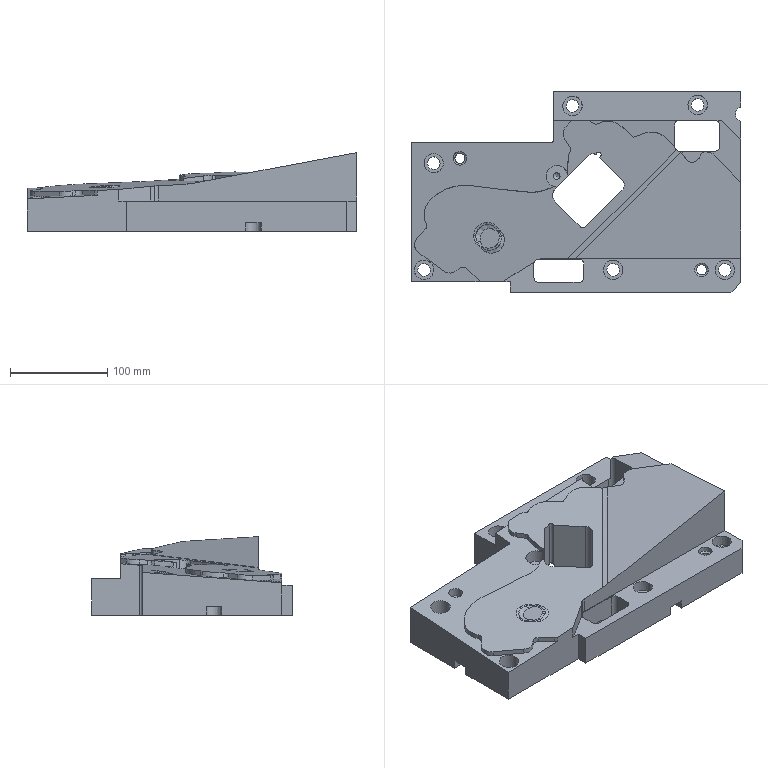Part | STEP file | gslz 2016.10.28-13_id1350_x_t | 1 solid | 171 faces | box 339.5 x 207 x 81.123 mm | volume 2655764 mm3 | plane 61 | cylinder 54 | spline 53 | cone 3 | commonest cylinder face diameters 10 x9 16 x7 20 x7 13 x6 14 x6 9 x5